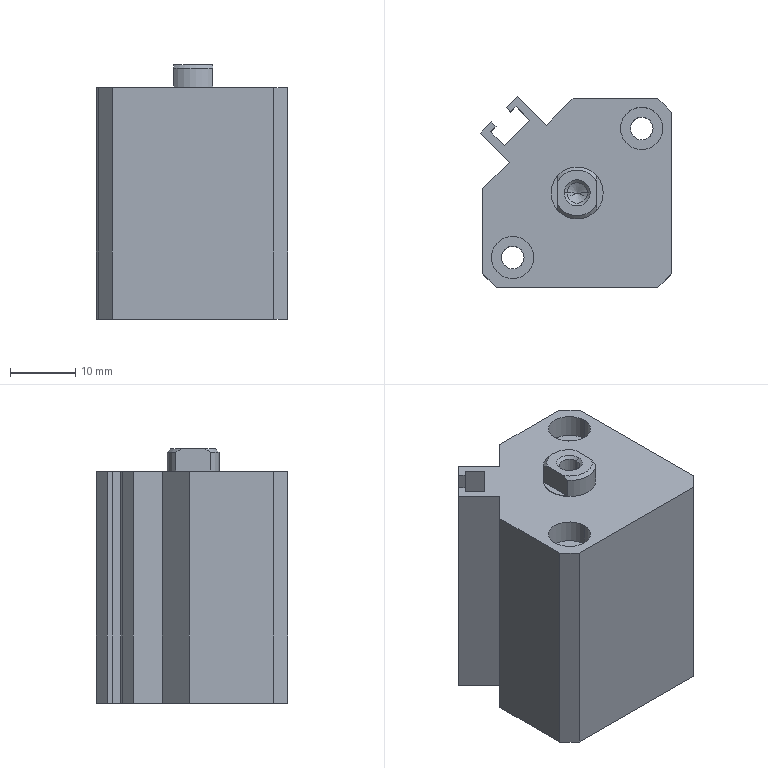Part | STEP file | CDQ2B16-5D | 1 solid | 63 faces | box 29.349 x 29.349 x 39 mm | volume 26194 mm3 | plane 33 | cylinder 20 | cone 10 | commonest cylinder face diameters 6.5 x8 3.5 x4 4.13 x4 3.14 x2 8 x2